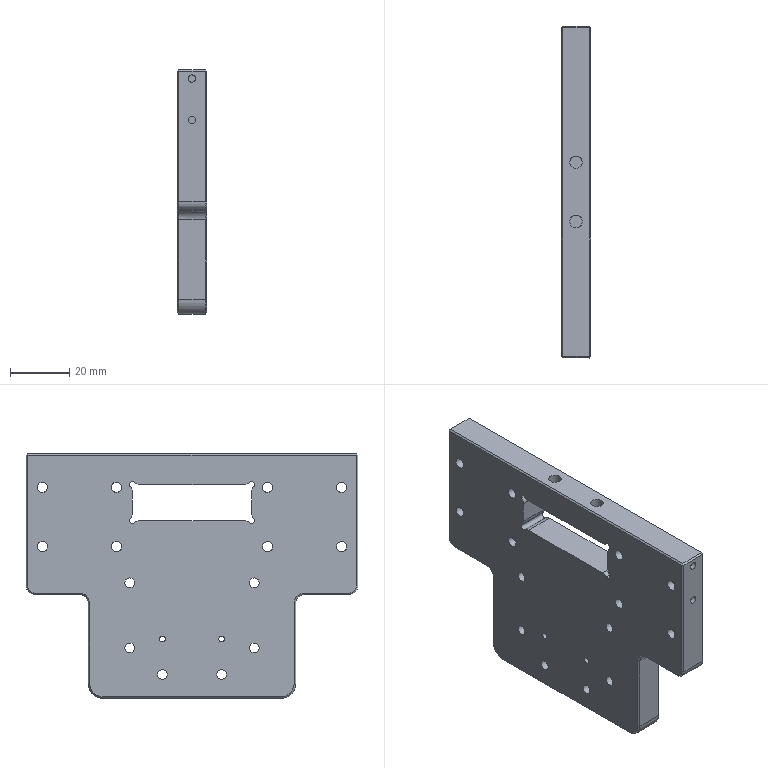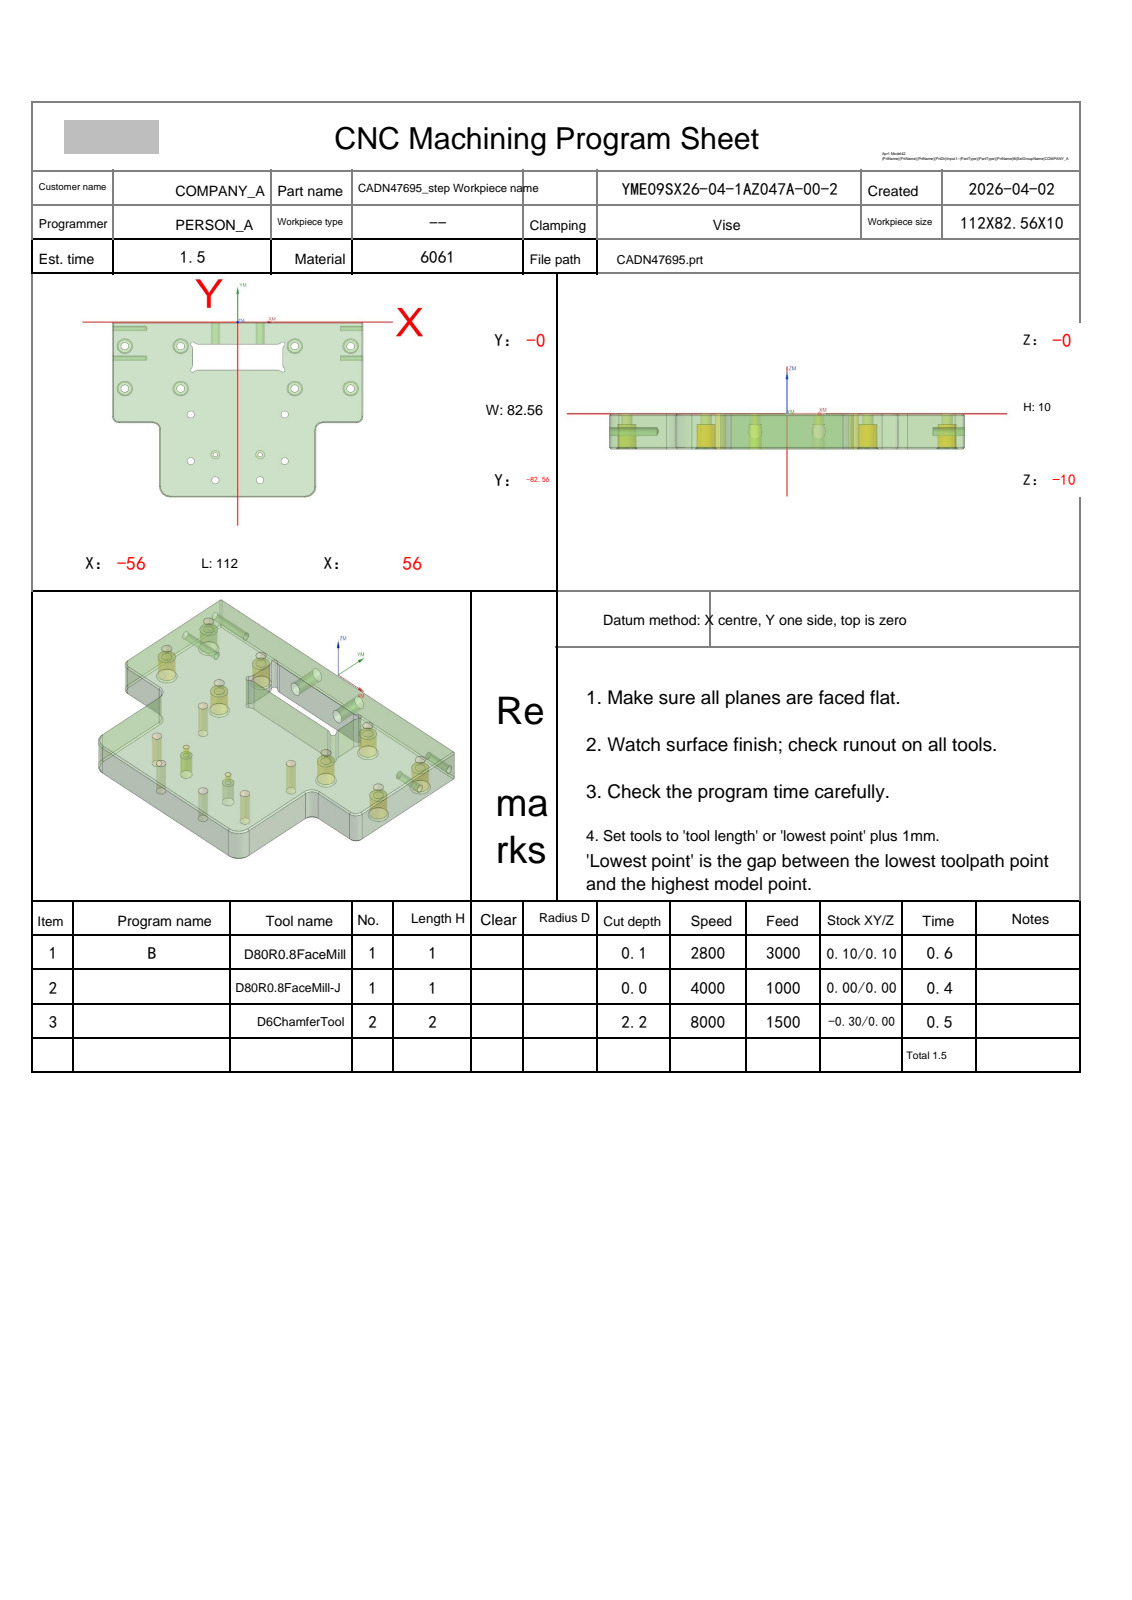NC program | NX | posted by the shop | part box 10 x 112 x 82.562 mm
Whole program:
%
O0001
(Machine time: 2.11 MIN)
(===Total Tool:2===)
(T1=D80R0.8 FaceMill D=80.  R=0.8  D-  H01 Z=-0.   )
(T2=D6ChamferTool   D=6.   R=0.   D-  H02 Z=-2.2  )
G80 G90 G17 G49 G40
G91 G28 Z0
M01
N1 T01 M06
(D80R0.8 FaceMill  D=80. R=0.8 H=01 ce=0.10 di=0.10)
G00 G90 G54 X106.263 Y-58.659 M03 S2800
G43 H01 Z20.
M08
Z3.525
G01 Z1.525 F3000.
X93.726
X-87.566
G02 X-95.441 Y-52.052 I.003 J8.
X-96.097 Y-44.562 I42.441 J7.489
G01 Y-39.261
G02 X-88.1 Y-31.263 I8. J-.003
G01 X96.097
X108.097
Z3.525
G00 X106.263 Y-58.659
Z3.05
G01 Z1.05
X93.726
X-87.566
G02 X-95.441 Y-52.052 I.003 J8.
X-96.097 Y-44.562 I42.441 J7.489
G01 Y-39.261
G02 X-88.1 Y-31.263 I8. J-.003
G01 X96.097
X108.097
Z3.05
G00 X106.263 Y-58.659
Z2.575
G01 Z.575
X93.726
X-87.566
G02 X-95.441 Y-52.052 I.003 J8.
X-96.097 Y-44.562 I42.441 J7.489
G01 Y-39.261
G02 X-88.1 Y-31.263 I8. J-.003
G01 X96.097
X108.097
Z2.575
G00 X106.263 Y-58.659
Z2.1
G01 Z.1
X93.726
X-87.566
G02 X-95.441 Y-52.052 I.003 J8.
X-96.097 Y-44.562 I42.441 J7.489
G01 Y-39.261
G02 X-88.1 Y-31.263 I8. J-.003
G01 X96.097
X108.097
Z2.1
G00 Z20.
G91 G28 Z0.0
M05
M09
G91 G28 Z0.0
M01
N2 T01 M06
(D80R0.8 FaceMill-J  D=80. R=0.8 H=01 ce=0.00 di=0.00)
G00 G90 G54 X106.413 Y-57.675 M03 S4000
G43 H01 Z20.
M08
Z2.
G01 Z0.0 F1000.
X93.904 Y-57.82
X-87.128 Y-59.916
X-87.218
G02 X-95.038 Y-53.6 I0.0 J8.
X-95.999 Y-44.562 I42.038 J9.038
G01 Y-39.737
G02 X-88.095 Y-31.741 I8. J-.003
G01 X95.999 Y-29.609
X107.999 Y-29.47
Z2.
G00 Z20.
G91 G28 Z0.0
M05
M09
G91 G28 Z0.0
M01
N3 T02 M06
(D6ChamferTool  D=6. R=0. H=02 ce=0.00 di=0.00)
G00 G90 G54 X10.008 Y-62.562 M03 S8000
G43 H02 Z20.
M08
G98 G81 X10.008 Y-62.562 Z-1.3 R3. F1000.
X-9.992
G80
G00 Z20.
G00 G90 X-50.5 Y-31.35 M03 S8000
Z20.
G98 G81 X-50.5 Y-31.35 Z-2.05 R3. F1000.
Y-11.35
X-25.5
Y-31.35
X25.5
Y-11.35
X50.5
Y-31.35
G80
G00 Z20.
G00 G90 X-21. Y-43.562 M03 S8000
Z20.
G98 G81 X-21. Y-43.562 Z-2.2 R3. F1000.
X-21.002 Y-65.562
X-10.003 Y-74.562
X9.997
X20.998 Y-65.562
Y-43.562
G80
G00 Z20.
G00 G90 X11.457 Y-21.9 M03 S7000
Z20.
Z2.5
G01 X17.789 Z.195 F1500.
X18.155 Y-21.937 Z.062
X18.514 Y-22.015 Z-.072
X18.861 Y-22.135 Z-.206
X19.193 Y-22.293 Z-.34
X19.504 Y-22.488 Z-.473
X19.791 Y-22.717 Z-.607
X19.92 Y-22.844 Z-.673
X20.016 Y-22.891 Z-.712
X20.123 Y-22.902 Z-.751
X20.226 Y-22.875 Z-.79
X20.314 Y-22.814 Z-.829
X20.375 Y-22.726 Z-.868
X20.402 Y-22.623 Z-.907
X20.391 Y-22.516 Z-.946
X20.344 Y-22.42 Z-.985
X20.314 Y-22.39 Z-1.
G02 X19.4 Y-20.151 I2.286 J2.24
G01 Y-12.849
G02 X20.314 Y-10.61 I3.2 J0.0
G03 X20.4 Y-10.4 I-.214 J.21
X20.1 Y-10.1 I-.3 J0.0
X19.89 Y-10.186 I0.0 J-.3
G02 X17.651 Y-11.1 I-2.24 J2.286
G01 X-17.651
G02 X-19.89 Y-10.186 I0.0 J3.2
G03 X-20.1 Y-10.1 I-.21 J-.214
X-20.4 Y-10.4 I0.0 J-.3
X-20.314 Y-10.61 I.3 J0.0
G02 X-19.4 Y-12.849 I-2.286 J-2.24
G01 Y-20.151
G02 X-20.314 Y-22.39 I-3.2 J0.0
G03 X-20.4 Y-22.6 I.214 J-.21
X-20.1 Y-22.9 I.3 J0.0
X-19.89 Y-22.814 I0.0 J.3
G02 X-17.651 Y-21.9 I2.24 J-2.286
G01 X17.651
G02 X19.89 Y-22.814 I0.0 J-3.2
G03 X20.1 Y-22.9 I.21 J.214
X20.4 Y-22.6 I0.0 J.3
X20.314 Y-22.39 I-.3 J0.0
G02 X19.994 Y-22.007 I2.286 J2.24
G01 Z1.5
G00 Z20.
G00 G90 X-17.716 Y-84.062 M03 S7000
Z20.
Z2.5
G01 X-30.079 Y-84.061 Z-2. F1500.
X-30.414 Y-84.049
X-30.917 Y-84.004
X-31.576 Y-83.876
X-32.219 Y-83.68
X-32.837 Y-83.42
X-33.426 Y-83.097
X-33.978 Y-82.715
X-34.488 Y-82.278
X-34.95 Y-81.791
X-35.36 Y-81.259
X-35.712 Y-80.688
X-36.004 Y-80.083
X-36.232 Y-79.451
X-36.393 Y-78.8
X-36.487 Y-78.135
X-36.505 Y-77.635
X-36.506 Y-77.562
Y-50.604
Y-50.565
G03 X-38.009 Y-49.062 I-1.503 J0.0
G01 X-38.048
X-53.
G02 X-57.5 Y-44.562 I0.0 J4.5
G01 Y-.5
G02 X-55.5 Y1.5 I2. J0.0
G01 X55.5
G02 X57.5 Y-.5 I0.0 J-2.
G01 Y-44.562
G02 X53. Y-49.062 I-4.5 J0.0
G01 X38.033
X37.994
G03 X36.493 Y-50.563 I0.0 J-1.501
G01 Y-50.602
Y-77.619
X36.49 Y-77.717
X36.476 Y-78.01
X36.435 Y-78.473
X36.307 Y-79.132
X36.111 Y-79.775
X35.851 Y-80.393
X35.528 Y-80.982
X35.146 Y-81.534
X34.709 Y-82.044
X34.222 Y-82.506
X33.69 Y-82.916
X33.119 Y-83.268
X32.514 Y-83.56
X31.883 Y-83.788
X31.231 Y-83.949
X30.566 Y-84.043
X30.066 Y-84.061
X29.993 Y-84.062
X-30.006
X-30.079 Y-84.061
X-30.414 Y-84.049
X-30.578 Y-84.034
Z.5
G00 Z20.
M05
M09
G91 G28 Z0.0
G91 G28 Y0.0
M30
%